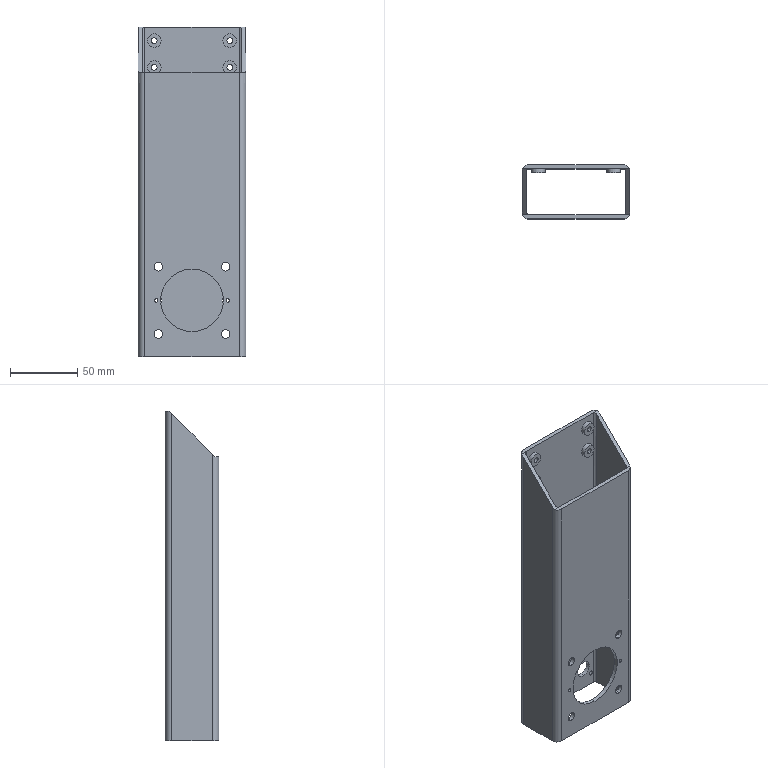Part | SolidWorks | features HoleWzd 5, ICE 4, Extrusion 1 | 1 solid | 75 faces | box 80 x 40 x 245 mm | volume 145168 mm3 | cylinder 58 | plane 17 | commonest cylinder face diameters 10 x12 3.3 x8 4.2 x8 6.5 x8 12 x8 2.5 x4